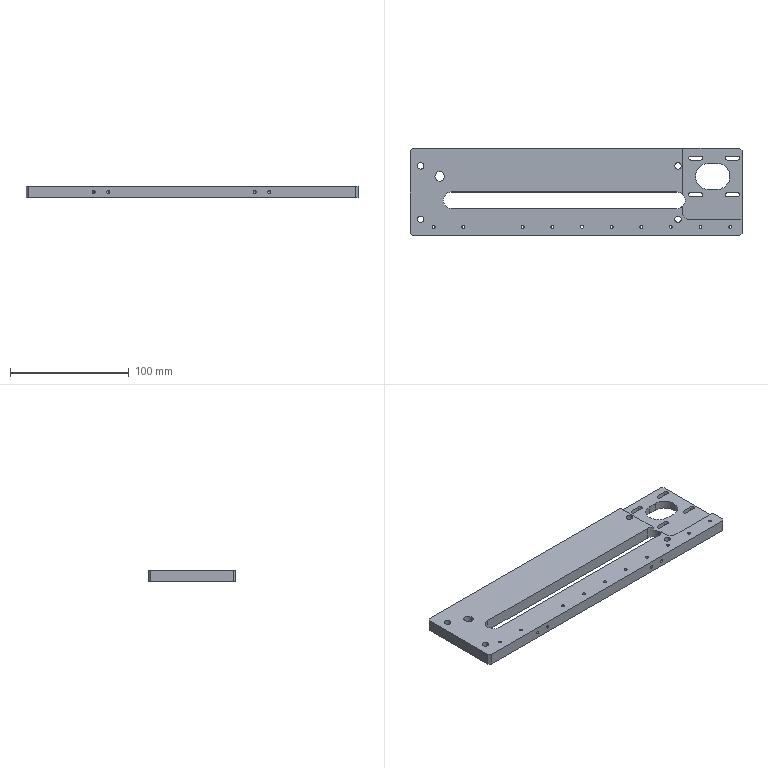Part | STEP file | FBDS-CS-022 | 1 solid | 120 faces | box 280 x 74 x 10 mm | volume 161210 mm3 | cylinder 75 | plane 31 | cone 14 | commonest cylinder face diameters 2.5 x32 3.4 x12 10 x9 5.5 x8 4.2 x6 14 x3